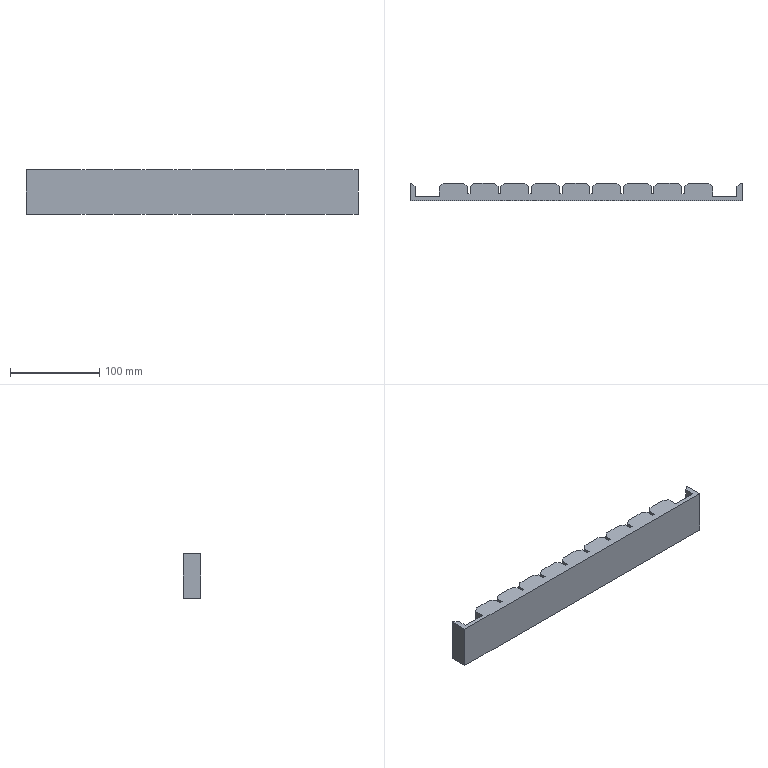CAM job | NX | 3-axis milling | part box 372.9 x 20 x 50 mm | stock box 378.9 x 20 x 50 mm
Tools:
number,name,description,diameter,corner_radius,flute_length,length,flutes
12,D6,Milling Tool-5 Parameters,6.0,0.0,50.0,75.0,2
16,D3,Milling Tool-5 Parameters,3.0,0.0,50.0,75.0,2
17,D3R0.5,Milling Tool-5 Parameters,3.0,0.5,50.0,75.0,2
Operations:
program,operation,operation_type,tool,method,geometry_group,spindle_rpm,surface_speed,feed_per_tooth,feed_cut,feed_plunge,cut_length_mm,path_length_mm,cut_time_min,machine_time_min
PROGRAM,FLOOR_WALL,VolumeBased25DMillingOperation,D6,METHOD,WORKPIECE,9500.0,179.0,0.1316,2500.0,100.0,22105.319,23243.912,8.842,8.956
PROGRAM,FLOOR_WALL_COPY,VolumeBased25DMillingOperation,D6,METHOD,WORKPIECE,9500.0,179.0,0.0632,1200.0,100.0,1114.965,1693.715,0.9291,0.987
PROGRAM,PLANAR_MILL,PlanarMilling,D3,METHOD,WORKPIECE,9500.0,89.0,0.0947,1800.0,100.0,19840.0,38302.85,11.022,12.868
PROGRAM,ZLEVEL_PROFILE,ZLevelMilling,D3R0.5,METHOD,WORKPIECE,9500.0,89.0,0.1316,2500.0,1000.0,45295.413,47511.178,18.145,18.367
PROGRAM,FLOOR_WALL_1,VolumeBased25DMillingOperation,D6,METHOD,WORKPIECE,9500.0,179.0,0.1316,2500.0,850.0,4728.708,9484.59,2.249,2.724
PROGRAM,FLOOR_WALL_1_COPY,VolumeBased25DMillingOperation,D6,METHOD,WORKPIECE,9500.0,179.0,0.0632,1200.0,850.0,139.08,711.58,0.1205,0.1778